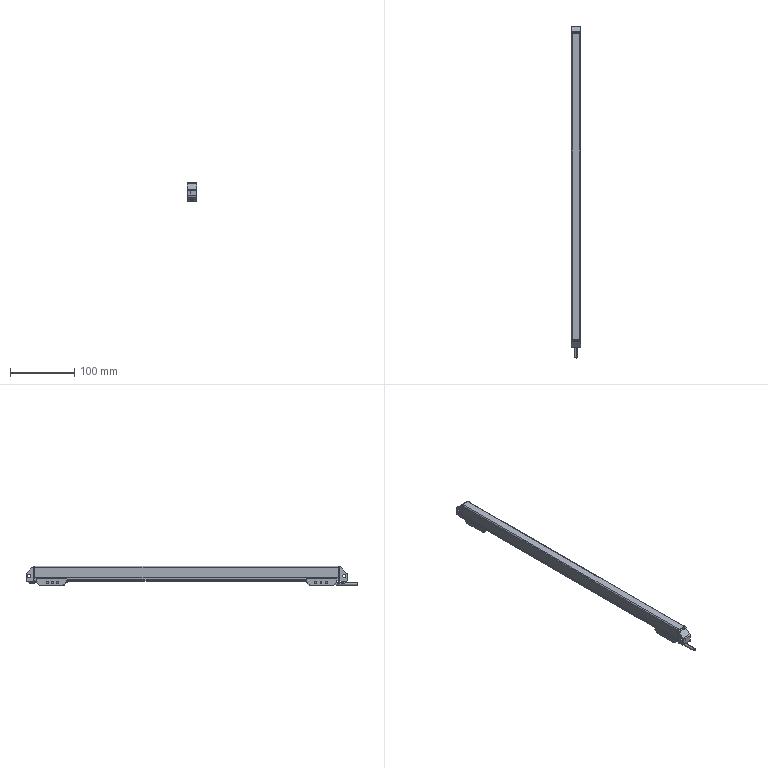Part | SolidWorks | features BaseBody 3 | 3 solids | 383 faces | box 15 x 516.175 x 30 mm | volume 163746 mm3 | plane 221 | cylinder 160 | spline 2 | commonest cylinder face diameters 2 x58 4 x50 1 x16 3 x12 0.4 x6 5 x4